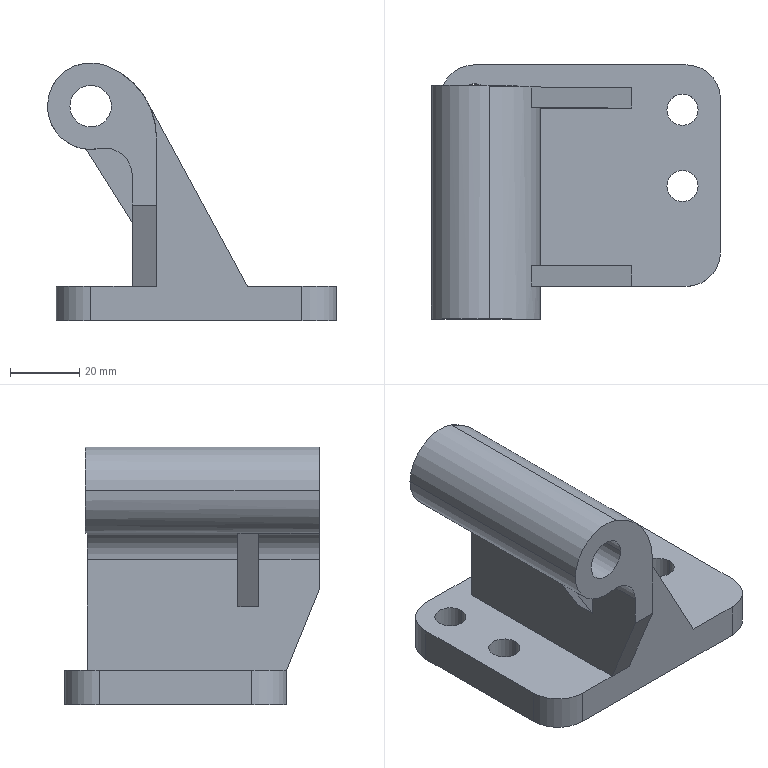Part | SolidWorks | features BaseBody 1 | 1 solid | 39 faces | box 83.5 x 73.5 x 74.5 mm | volume 109761 mm3 | plane 20 | cylinder 19 | commonest cylinder face diameters 9 x8 20 x4 12 x2 16 x2 25 x2 44.504 x1
STEP:
#1=CARTESIAN_POINT('',(5.5,32.,10.));
#2=VERTEX_POINT('',#1);
#3=CARTESIAN_POINT('',(14.5,32.,10.));
#4=VERTEX_POINT('',#3);
#5=CARTESIAN_POINT('',(10.,32.,10.));
#6=DIRECTION('',(0.,0.,-1.));
#7=DIRECTION('',(-1.,0.,0.));
#8=AXIS2_PLACEMENT_3D('',#5,#6,#7);
#9=CIRCLE('',#8,4.5);
#10=EDGE_CURVE('',#2,#4,#9,.T.);
#11=ORIENTED_EDGE('',*,*,#10,.F.);
#12=CARTESIAN_POINT('',(5.5,32.,0.));
#13=VERTEX_POINT('',#12);
#14=CARTESIAN_POINT('',(5.5,32.,10.));
#15=DIRECTION('',(0.,0.,-1.));
#16=VECTOR('',#15,1000.);
#17=LINE('',#14,#16);
#18=EDGE_CURVE('',#2,#13,#17,.T.);
#19=ORIENTED_EDGE('',*,*,#18,.T.);
#20=CARTESIAN_POINT('',(14.5,32.,0.));
#21=VERTEX_POINT('',#20);
#22=CARTESIAN_POINT('',(10.,32.,0.));
#23=DIRECTION('',(0.,0.,-1.));
#24=DIRECTION('',(-1.,0.,0.));
#25=AXIS2_PLACEMENT_3D('',#22,#23,#24);
#26=CIRCLE('',#25,4.5);
#27=EDGE_CURVE('',#13,#21,#26,.T.);
#28=ORIENTED_EDGE('',*,*,#27,.T.);
#29=CARTESIAN_POINT('',(14.5,32.,10.));
#30=DIRECTION('',(0.,0.,-1.));
#31=VECTOR('',#30,1000.);
#32=LINE('',#29,#31);
#33=EDGE_CURVE('',#4,#21,#32,.T.);
#34=ORIENTED_EDGE('',*,*,#33,.F.);
#35=EDGE_LOOP('',(#11,#19,#28,#34));
#36=FACE_OUTER_BOUND('',#35,.T.);
#37=CARTESIAN_POINT('',(10.,32.,10.));
#38=DIRECTION('',(0.,0.,-1.));
#39=DIRECTION('',(1.,0.,0.));
#40=AXIS2_PLACEMENT_3D('',#37,#38,#39);
#41=CYLINDRICAL_SURFACE('',#40,4.5);
#42=ADVANCED_FACE('',(#36),#41,.F.);
#43=CARTESIAN_POINT('',(5.5,54.,10.));
#44=VERTEX_POINT('',#43);
#45=CARTESIAN_POINT('',(14.5,54.,10.));
#46=VERTEX_POINT('',#45);
#47=CARTESIAN_POINT('',(10.,54.,10.));
#48=DIRECTION('',(0.,0.,-1.));
#49=DIRECTION('',(-1.,0.,0.));
#50=AXIS2_PLACEMENT_3D('',#47,#48,#49);
#51=CIRCLE('',#50,4.5);
#52=EDGE_CURVE('',#44,#46,#51,.T.);
#53=ORIENTED_EDGE('',*,*,#52,.F.);
#54=CARTESIAN_POINT('',(5.5,54.,0.));
#55=VERTEX_POINT('',#54);
#56=CARTESIAN_POINT('',(5.5,54.,10.));
#57=DIRECTION('',(0.,0.,-1.));
#58=VECTOR('',#57,1000.);
#59=LINE('',#56,#58);
#60=EDGE_CURVE('',#44,#55,#59,.T.);
#61=ORIENTED_EDGE('',*,*,#60,.T.);
#62=CARTESIAN_POINT('',(14.5,54.,0.));
#63=VERTEX_POINT('',#62);
#64=CARTESIAN_POINT('',(10.,54.,0.));
#65=DIRECTION('',(0.,0.,-1.));
#66=DIRECTION('',(-1.,0.,0.));
#67=AXIS2_PLACEMENT_3D('',#64,#65,#66);
#68=CIRCLE('',#67,4.5);
#69=EDGE_CURVE('',#55,#63,#68,.T.);
#70=ORIENTED_EDGE('',*,*,#69,.T.);
#71=CARTESIAN_POINT('',(14.5,54.,10.));
#72=DIRECTION('',(0.,0.,-1.));
#73=VECTOR('',#72,1000.);
#74=LINE('',#71,#73);
#75=EDGE_CURVE('',#46,#63,#74,.T.);
#76=ORIENTED_EDGE('',*,*,#75,.F.);
#77=EDGE_LOOP('',(#53,#61,#70,#76));
#78=FACE_OUTER_BOUND('',#77,.T.);
#79=CARTESIAN_POINT('',(10.,54.,10.));
#80=DIRECTION('',(0.,0.,-1.));
#81=DIRECTION('',(1.,0.,0.));
#82=AXIS2_PLACEMENT_3D('',#79,#80,#81);
#83=CYLINDRICAL_SURFACE('',#82,4.5);
#84=ADVANCED_FACE('',(#78),#83,.F.);
#85=CARTESIAN_POINT('',(22.5,58.,62.));
#86=VERTEX_POINT('',#85);
#87=CARTESIAN_POINT('',(-2.5,58.,62.));
#88=VERTEX_POINT('',#87);
#89=CARTESIAN_POINT('',(10.,58.,62.));
#90=DIRECTION('',(0.,1.,0.));
#91=DIRECTION('',(0.,0.,-1.));
#92=AXIS2_PLACEMENT_3D('',#89,#90,#91);
#93=CIRCLE('',#92,12.5);
#94=EDGE_CURVE('',#86,#88,#93,.T.);
#95=ORIENTED_EDGE('',*,*,#94,.F.);
#96=CARTESIAN_POINT('',(22.5,57.5,62.));
#97=VERTEX_POINT('',#96);
#98=CARTESIAN_POINT('',(22.5,57.5,62.));
#99=DIRECTION('',(0.,-1.,0.));
#100=VECTOR('',#99,1000.);
#101=LINE('',#98,#100);
#102=EDGE_CURVE('',#86,#97,#101,.T.);
#103=ORIENTED_EDGE('',*,*,#102,.T.);
#104=CARTESIAN_POINT('',(12.439,57.5,49.74));
#105=VERTEX_POINT('',#104);
#106=CARTESIAN_POINT('',(10.,57.5,62.));
#107=DIRECTION('',(0.,-1.,0.));
#108=DIRECTION('',(0.,0.,-1.));
#109=AXIS2_PLACEMENT_3D('',#106,#107,#108);
#110=CIRCLE('',#109,12.5);
#111=EDGE_CURVE('',#105,#97,#110,.T.);
#112=ORIENTED_EDGE('',*,*,#111,.F.);
#113=CARTESIAN_POINT('',(12.439,14.,49.74));
#114=VERTEX_POINT('',#113);
#115=CARTESIAN_POINT('',(12.439,-9.5,49.74));
#116=DIRECTION('',(0.,1.,0.));
#117=VECTOR('',#116,1000.);
#118=LINE('',#115,#117);
#119=EDGE_CURVE('',#114,#105,#118,.T.);
#120=ORIENTED_EDGE('',*,*,#119,.F.);
#121=CARTESIAN_POINT('',(8.698,14.,49.568));
#122=VERTEX_POINT('',#121);
#123=CARTESIAN_POINT('',(10.,14.,62.));
#124=DIRECTION('',(0.,-1.,0.));
#125=DIRECTION('',(0.,0.,1.));
#126=AXIS2_PLACEMENT_3D('',#123,#124,#125);
#127=CIRCLE('',#126,12.5);
#128=EDGE_CURVE('',#122,#114,#127,.T.);
#129=ORIENTED_EDGE('',*,*,#128,.F.);
#130=CARTESIAN_POINT('',(8.698,8.,49.568));
#131=VERTEX_POINT('',#130);
#132=CARTESIAN_POINT('',(8.698,57.5,49.568));
#133=DIRECTION('',(0.,-1.,0.));
#134=VECTOR('',#133,1000.);
#135=LINE('',#132,#134);
#136=EDGE_CURVE('',#122,#131,#135,.T.);
#137=ORIENTED_EDGE('',*,*,#136,.T.);
#138=CARTESIAN_POINT('',(12.439,8.,49.74));
#139=VERTEX_POINT('',#138);
#140=CARTESIAN_POINT('',(10.,8.,62.));
#141=DIRECTION('',(0.,-1.,0.));
#142=DIRECTION('',(0.,0.,1.));
#143=AXIS2_PLACEMENT_3D('',#140,#141,#142);
#144=CIRCLE('',#143,12.5);
#145=EDGE_CURVE('',#131,#139,#144,.T.);
#146=ORIENTED_EDGE('',*,*,#145,.T.);
#147=CARTESIAN_POINT('',(12.439,-9.5,49.74));
#148=VERTEX_POINT('',#147);
#149=CARTESIAN_POINT('',(12.439,-9.5,49.74));
#150=DIRECTION('',(0.,1.,0.));
#151=VECTOR('',#150,1000.);
#152=LINE('',#149,#151);
#153=EDGE_CURVE('',#148,#139,#152,.T.);
#154=ORIENTED_EDGE('',*,*,#153,.F.);
#155=CARTESIAN_POINT('',(-2.5,-9.5,62.));
#156=VERTEX_POINT('',#155);
#157=CARTESIAN_POINT('',(10.,-9.5,62.));
#158=DIRECTION('',(0.,1.,0.));
#159=DIRECTION('',(0.,0.,1.));
#160=AXIS2_PLACEMENT_3D('',#157,#158,#159);
#161=CIRCLE('',#160,12.5);
#162=EDGE_CURVE('',#148,#156,#161,.T.);
#163=ORIENTED_EDGE('',*,*,#162,.T.);
#164=CARTESIAN_POINT('',(-2.5,57.5,62.));
#165=DIRECTION('',(0.,-1.,0.));
#166=VECTOR('',#165,1000.);
#167=LINE('',#164,#166);
#168=EDGE_CURVE('',#88,#156,#167,.T.);
#169=ORIENTED_EDGE('',*,*,#168,.F.);
#170=EDGE_LOOP('',(#95,#103,#112,#120,#129,#137,#146,#154,#163,#169));
#171=FACE_OUTER_BOUND('',#170,.T.);
#172=CARTESIAN_POINT('',(10.,57.5,62.));
#173=DIRECTION('',(0.,-1.,0.));
#174=DIRECTION('',(-1.,0.,0.));
#175=AXIS2_PLACEMENT_3D('',#172,#173,#174);
#176=CYLINDRICAL_SURFACE('',#175,12.5);
#177=ADVANCED_FACE('',(#171),#176,.T.);
#178=CARTESIAN_POINT('',(4.,58.,62.));
#179=VERTEX_POINT('',#178);
#180=CARTESIAN_POINT('',(16.,58.,62.));
#181=VERTEX_POINT('',#180);
#182=CARTESIAN_POINT('',(10.,58.,62.));
#183=DIRECTION('',(0.,1.,0.));
#184=DIRECTION('',(0.,0.,-1.));
#185=AXIS2_PLACEMENT_3D('',#182,#183,#184);
#186=CIRCLE('',#185,6.);
#187=EDGE_CURVE('',#179,#181,#186,.T.);
#188=ORIENTED_EDGE('',*,*,#187,.T.);
#189=CARTESIAN_POINT('',(16.,-9.5,62.));
#190=VERTEX_POINT('',#189);
#191=CARTESIAN_POINT('',(16.,57.5,62.));
#192=DIRECTION('',(0.,-1.,0.));
#193=VECTOR('',#192,1000.);
#194=LINE('',#191,#193);
#195=EDGE_CURVE('',#181,#190,#194,.T.);
#196=ORIENTED_EDGE('',*,*,#195,.T.);
#197=CARTESIAN_POINT('',(4.,-9.5,62.));
#198=VERTEX_POINT('',#197);
#199=CARTESIAN_POINT('',(10.,-9.5,62.));
#200=DIRECTION('',(0.,1.,0.));
#201=DIRECTION('',(0.,0.,1.));
#202=AXIS2_PLACEMENT_3D('',#199,#200,#201);
#203=CIRCLE('',#202,6.);
#204=EDGE_CURVE('',#198,#190,#203,.T.);
#205=ORIENTED_EDGE('',*,*,#204,.F.);
#206=CARTESIAN_POINT('',(4.,57.5,62.));
#207=DIRECTION('',(0.,-1.,0.));
#208=VECTOR('',#207,1000.);
#209=LINE('',#206,#208);
#210=EDGE_CURVE('',#179,#198,#209,.T.);
#211=ORIENTED_EDGE('',*,*,#210,.F.);
#212=EDGE_LOOP('',(#188,#196,#205,#211));
#213=FACE_OUTER_BOUND('',#212,.T.);
#214=CARTESIAN_POINT('',(10.,57.5,62.));
#215=DIRECTION('',(0.,-1.,0.));
#216=DIRECTION('',(-1.,0.,0.));
#217=AXIS2_PLACEMENT_3D('',#214,#215,#216);
#218=CYLINDRICAL_SURFACE('',#217,6.);
#219=ADVANCED_FACE('',(#213),#218,.F.);
#220=CARTESIAN_POINT('',(65.5,29.,10.));
#221=VERTEX_POINT('',#220);
#222=CARTESIAN_POINT('',(74.5,29.,10.));
#223=VERTEX_POINT('',#222);
#224=CARTESIAN_POINT('',(70.,29.,10.));
#225=DIRECTION('',(0.,0.,-1.));
#226=DIRECTION('',(-1.,0.,0.));
#227=AXIS2_PLACEMENT_3D('',#224,#225,#226);
#228=CIRCLE('',#227,4.5);
#229=EDGE_CURVE('',#221,#223,#228,.T.);
#230=ORIENTED_EDGE('',*,*,#229,.F.);
#231=CARTESIAN_POINT('',(65.5,29.,0.));
#232=VERTEX_POINT('',#231);
#233=CARTESIAN_POINT('',(65.5,29.,20.));
#234=DIRECTION('',(0.,0.,-1.));
#235=VECTOR('',#234,1000.);
#236=LINE('',#233,#235);
#237=EDGE_CURVE('',#221,#232,#236,.T.);
#238=ORIENTED_EDGE('',*,*,#237,.T.);
#239=CARTESIAN_POINT('',(74.5,29.,0.));
#240=VERTEX_POINT('',#239);
#241=CARTESIAN_POINT('',(70.,29.,0.));
#242=DIRECTION('',(0.,0.,-1.));
#243=DIRECTION('',(-1.,0.,0.));
#244=AXIS2_PLACEMENT_3D('',#241,#242,#243);
#245=CIRCLE('',#244,4.5);
#246=EDGE_CURVE('',#232,#240,#245,.T.);
#247=ORIENTED_EDGE('',*,*,#246,.T.);
#248=CARTESIAN_POINT('',(74.5,29.,20.));
#249=DIRECTION('',(0.,0.,-1.));
#250=VECTOR('',#249,1000.);
#251=LINE('',#248,#250);
#252=EDGE_CURVE('',#223,#240,#251,.T.);
#253=ORIENTED_EDGE('',*,*,#252,.F.);
#254=EDGE_LOOP('',(#230,#238,#247,#253));
#255=FACE_OUTER_BOUND('',#254,.T.);
#256=CARTESIAN_POINT('',(70.,29.,20.));
#257=DIRECTION('',(0.,0.,-1.));
#258=DIRECTION('',(1.,0.,0.));
#259=AXIS2_PLACEMENT_3D('',#256,#257,#258);
#260=CYLINDRICAL_SURFACE('',#259,4.5);
#261=ADVANCED_FACE('',(#255),#260,.F.);
#262=CARTESIAN_POINT('',(65.5,51.,10.));
#263=VERTEX_POINT('',#262);
#264=CARTESIAN_POINT('',(74.5,51.,10.));
#265=VERTEX_POINT('',#264);
#266=CARTESIAN_POINT('',(70.,51.,10.));
#267=DIRECTION('',(0.,0.,-1.));
#268=DIRECTION('',(-1.,0.,0.));
#269=AXIS2_PLACEMENT_3D('',#266,#267,#268);
#270=CIRCLE('',#269,4.5);
#271=EDGE_CURVE('',#263,#265,#270,.T.);
#272=ORIENTED_EDGE('',*,*,#271,.F.);
#273=CARTESIAN_POINT('',(65.5,51.,0.));
#274=VERTEX_POINT('',#273);
#275=CARTESIAN_POINT('',(65.5,51.,20.));
#276=DIRECTION('',(0.,0.,-1.));
#277=VECTOR('',#276,1000.);
#278=LINE('',#275,#277);
#279=EDGE_CURVE('',#263,#274,#278,.T.);
#280=ORIENTED_EDGE('',*,*,#279,.T.);
#281=CARTESIAN_POINT('',(74.5,51.,0.));
#282=VERTEX_POINT('',#281);
#283=CARTESIAN_POINT('',(70.,51.,0.));
#284=DIRECTION('',(0.,0.,-1.));
#285=DIRECTION('',(-1.,0.,0.));
#286=AXIS2_PLACEMENT_3D('',#283,#284,#285);
#287=CIRCLE('',#286,4.5);
#288=EDGE_CURVE('',#274,#282,#287,.T.);
#289=ORIENTED_EDGE('',*,*,#288,.T.);
#290=CARTESIAN_POINT('',(74.5,51.,20.));
#291=DIRECTION('',(0.,0.,-1.));
#292=VECTOR('',#291,1000.);
#293=LINE('',#290,#292);
#294=EDGE_CURVE('',#265,#282,#293,.T.);
#295=ORIENTED_EDGE('',*,*,#294,.F.);
#296=EDGE_LOOP('',(#272,#280,#289,#295));
#297=FACE_OUTER_BOUND('',#296,.T.);
#298=CARTESIAN_POINT('',(70.,51.,20.));
#299=DIRECTION('',(0.,0.,-1.));
#300=DIRECTION('',(1.,0.,0.));
#301=AXIS2_PLACEMENT_3D('',#298,#299,#300);
#302=CYLINDRICAL_SURFACE('',#301,4.5);
#303=ADVANCED_FACE('',(#297),#302,.F.);
#304=ORIENTED_EDGE('',*,*,#187,.F.);
#305=CARTESIAN_POINT('',(10.,58.,62.));
#306=DIRECTION('',(0.,1.,0.));
#307=DIRECTION('',(0.,0.,-1.));
#308=AXIS2_PLACEMENT_3D('',#305,#306,#307);
#309=CIRCLE('',#308,6.);
#310=EDGE_CURVE('',#181,#179,#309,.T.);
#311=ORIENTED_EDGE('',*,*,#310,.F.);
#312=EDGE_LOOP('',(#304,#311));
#313=FACE_BOUND('',#312,.T.);
#314=CARTESIAN_POINT('',(10.,58.,62.));
#315=DIRECTION('',(0.,1.,0.));
#316=DIRECTION('',(0.,0.,-1.));
#317=AXIS2_PLACEMENT_3D('',#314,#315,#316);
#318=CIRCLE('',#317,12.5);
#319=EDGE_CURVE('',#88,#86,#318,.T.);
#320=ORIENTED_EDGE('',*,*,#319,.T.);
#321=ORIENTED_EDGE('',*,*,#94,.T.);
#322=EDGE_LOOP('',(#320,#321));
#323=FACE_OUTER_BOUND('',#322,.T.);
#324=CARTESIAN_POINT('',(10.,58.,62.));
#325=DIRECTION('',(0.,1.,0.));
#326=DIRECTION('',(1.,0.,0.));
#327=AXIS2_PLACEMENT_3D('',#324,#325,#326);
#328=PLANE('',#327);
#329=ADVANCED_FACE('',(#313,#323),#328,.T.);
#330=CARTESIAN_POINT('',(81.,54.,10.));
#331=VERTEX_POINT('',#330);
#332=CARTESIAN_POINT('',(71.,64.,10.));
#333=VERTEX_POINT('',#332);
#334=CARTESIAN_POINT('',(71.,54.,10.));
#335=DIRECTION('',(0.,0.,1.));
#336=DIRECTION('',(-1.,0.,0.));
#337=AXIS2_PLACEMENT_3D('',#334,#335,#336);
#338=CIRCLE('',#337,10.);
#339=EDGE_CURVE('',#331,#333,#338,.T.);
#340=ORIENTED_EDGE('',*,*,#339,.F.);
#341=CARTESIAN_POINT('',(81.,54.,0.));
#342=VERTEX_POINT('',#341);
#343=CARTESIAN_POINT('',(81.,54.,10.));
#344=DIRECTION('',(0.,0.,1.));
#345=VECTOR('',#344,1000.);
#346=LINE('',#343,#345);
#347=EDGE_CURVE('',#342,#331,#346,.T.);
#348=ORIENTED_EDGE('',*,*,#347,.F.);
#349=CARTESIAN_POINT('',(71.,64.,0.));
#350=VERTEX_POINT('',#349);
#351=CARTESIAN_POINT('',(71.,54.,0.));
#352=DIRECTION('',(0.,0.,-1.));
#353=DIRECTION('',(-1.,0.,0.));
#354=AXIS2_PLACEMENT_3D('',#351,#352,#353);
#355=CIRCLE('',#354,10.);
#356=EDGE_CURVE('',#350,#342,#355,.T.);
#357=ORIENTED_EDGE('',*,*,#356,.F.);
#358=CARTESIAN_POINT('',(71.,64.,10.));
#359=DIRECTION('',(0.,0.,-1.));
#360=VECTOR('',#359,1000.);
#361=LINE('',#358,#360);
#362=EDGE_CURVE('',#333,#350,#361,.T.);
#363=ORIENTED_EDGE('',*,*,#362,.F.);
#364=EDGE_LOOP('',(#340,#348,#357,#363));
#365=FACE_OUTER_BOUND('',#364,.T.);
#366=CARTESIAN_POINT('',(71.,54.,10.));
#367=DIRECTION('',(0.,0.,-1.));
#368=DIRECTION('',(1.,0.,0.));
#369=AXIS2_PLACEMENT_3D('',#366,#367,#368);
#370=CYLINDRICAL_SURFACE('',#369,10.);
#371=ADVANCED_FACE('',(#365),#370,.T.);
#372=CARTESIAN_POINT('',(71.,0.,10.));
#373=VERTEX_POINT('',#372);
#374=CARTESIAN_POINT('',(81.,10.,10.));
#375=VERTEX_POINT('',#374);
#376=CARTESIAN_POINT('',(71.,10.,10.));
#377=DIRECTION('',(0.,0.,1.));
#378=DIRECTION('',(-1.,0.,0.));
#379=AXIS2_PLACEMENT_3D('',#376,#377,#378);
#380=CIRCLE('',#379,10.);
#381=EDGE_CURVE('',#373,#375,#380,.T.);
#382=ORIENTED_EDGE('',*,*,#381,.F.);
#383=CARTESIAN_POINT('',(71.,0.,0.));
#384=VERTEX_POINT('',#383);
#385=CARTESIAN_POINT('',(71.,0.,10.));
#386=DIRECTION('',(0.,0.,1.));
#387=VECTOR('',#386,1000.);
#388=LINE('',#385,#387);
#389=EDGE_CURVE('',#384,#373,#388,.T.);
#390=ORIENTED_EDGE('',*,*,#389,.F.);
#391=CARTESIAN_POINT('',(81.,10.,0.));
#392=VERTEX_POINT('',#391);
#393=CARTESIAN_POINT('',(71.,10.,0.));
#394=DIRECTION('',(0.,0.,-1.));
#395=DIRECTION('',(-1.,0.,0.));
#396=AXIS2_PLACEMENT_3D('',#393,#394,#395);
#397=CIRCLE('',#396,10.);
#398=EDGE_CURVE('',#392,#384,#397,.T.);
#399=ORIENTED_EDGE('',*,*,#398,.F.);
#400=CARTESIAN_POINT('',(81.,10.,10.));
#401=DIRECTION('',(0.,0.,-1.));
#402=VECTOR('',#401,1000.);
#403=LINE('',#400,#402);
#404=EDGE_CURVE('',#375,#392,#403,.T.);
#405=ORIENTED_EDGE('',*,*,#404,.F.);
#406=EDGE_LOOP('',(#382,#390,#399,#405));
#407=FACE_OUTER_BOUND('',#406,.T.);
#408=CARTESIAN_POINT('',(71.,10.,10.));
#409=DIRECTION('',(0.,0.,-1.));
#410=DIRECTION('',(1.,0.,0.));
#411=AXIS2_PLACEMENT_3D('',#408,#409,#410);
#412=CYLINDRICAL_SURFACE('',#411,10.);
#413=ADVANCED_FACE('',(#407),#412,.T.);
#414=CARTESIAN_POINT('',(10.,64.,10.));
#415=VERTEX_POINT('',#414);
#416=CARTESIAN_POINT('',(0.,54.,10.));
#417=VERTEX_POINT('',#416);
#418=CARTESIAN_POINT('',(10.,54.,10.));
#419=DIRECTION('',(0.,0.,1.));
#420=DIRECTION('',(-1.,0.,0.));
#421=AXIS2_PLACEMENT_3D('',#418,#419,#420);
#422=CIRCLE('',#421,10.);
#423=EDGE_CURVE('',#415,#417,#422,.T.);
#424=ORIENTED_EDGE('',*,*,#423,.F.);
#425=CARTESIAN_POINT('',(10.,64.,0.));
#426=VERTEX_POINT('',#425);
#427=CARTESIAN_POINT('',(10.,64.,10.));
#428=DIRECTION('',(0.,0.,1.));
#429=VECTOR('',#428,1000.);
#430=LINE('',#427,#429);
#431=EDGE_CURVE('',#426,#415,#430,.T.);
#432=ORIENTED_EDGE('',*,*,#431,.F.);
#433=CARTESIAN_POINT('',(0.,54.,0.));
#434=VERTEX_POINT('',#433);
#435=CARTESIAN_POINT('',(10.,54.,0.));
#436=DIRECTION('',(0.,0.,-1.));
#437=DIRECTION('',(-1.,0.,0.));
#438=AXIS2_PLACEMENT_3D('',#435,#436,#437);
#439=CIRCLE('',#438,10.);
#440=EDGE_CURVE('',#434,#426,#439,.T.);
#441=ORIENTED_EDGE('',*,*,#440,.F.);
#442=CARTESIAN_POINT('',(0.,54.,10.));
#443=DIRECTION('',(0.,0.,-1.));
#444=VECTOR('',#443,1000.);
#445=LINE('',#442,#444);
#446=EDGE_CURVE('',#417,#434,#445,.T.);
#447=ORIENTED_EDGE('',*,*,#446,.F.);
#448=EDGE_LOOP('',(#424,#432,#441,#447));
#449=FACE_OUTER_BOUND('',#448,.T.);
#450=CARTESIAN_POINT('',(10.,54.,10.));
#451=DIRECTION('',(0.,0.,-1.));
#452=DIRECTION('',(1.,0.,0.));
#453=AXIS2_PLACEMENT_3D('',#450,#451,#452);
#454=CYLINDRICAL_SURFACE('',#453,10.);
#455=ADVANCED_FACE('',(#449),#454,.T.);
#456=CARTESIAN_POINT('',(0.,10.,10.));
#457=VERTEX_POINT('',#456);
#458=CARTESIAN_POINT('',(10.,0.,10.));
#459=VERTEX_POINT('',#458);
#460=CARTESIAN_POINT('',(10.,10.,10.));
#461=DIRECTION('',(0.,0.,1.));
#462=DIRECTION('',(-1.,0.,0.));
#463=AXIS2_PLACEMENT_3D('',#460,#461,#462);
#464=CIRCLE('',#463,10.);
#465=EDGE_CURVE('',#457,#459,#464,.T.);
#466=ORIENTED_EDGE('',*,*,#465,.F.);
#467=CARTESIAN_POINT('',(0.,10.,0.));
#468=VERTEX_POINT('',#467);
#469=CARTESIAN_POINT('',(0.,10.,10.));
#470=DIRECTION('',(0.,0.,1.));
#471=VECTOR('',#470,1000.);
#472=LINE('',#469,#471);
#473=EDGE_CURVE('',#468,#457,#472,.T.);
#474=ORIENTED_EDGE('',*,*,#473,.F.);
#475=CARTESIAN_POINT('',(10.,0.,0.));
#476=VERTEX_POINT('',#475);
#477=CARTESIAN_POINT('',(10.,10.,0.));
#478=DIRECTION('',(0.,0.,-1.));
#479=DIRECTION('',(-1.,0.,0.));
#480=AXIS2_PLACEMENT_3D('',#477,#478,#479);
#481=CIRCLE('',#480,10.);
#482=EDGE_CURVE('',#476,#468,#481,.T.);
#483=ORIENTED_EDGE('',*,*,#482,.F.);
#484=CARTESIAN_POINT('',(10.,0.,10.));
#485=DIRECTION('',(0.,0.,-1.));
#486=VECTOR('',#485,1000.);
#487=LINE('',#484,#486);
#488=EDGE_CURVE('',#459,#476,#487,.T.);
#489=ORIENTED_EDGE('',*,*,#488,.F.);
#490=EDGE_LOOP('',(#466,#474,#483,#489));
#491=FACE_OUTER_BOUND('',#490,.T.);
#492=CARTESIAN_POINT('',(10.,10.,10.));
#493=DIRECTION('',(0.,0.,-1.));
#494=DIRECTION('',(1.,0.,0.));
#495=AXIS2_PLACEMENT_3D('',#492,#493,#494);
#496=CYLINDRICAL_SURFACE('',#495,10.);
#497=ADVANCED_FACE('',(#491),#496,.T.);
#498=ORIENTED_EDGE('',*,*,#279,.F.);
#499=CARTESIAN_POINT('',(70.,51.,10.));
#500=DIRECTION('',(0.,0.,-1.));
#501=DIRECTION('',(-1.,0.,0.));
#502=AXIS2_PLACEMENT_3D('',#499,#500,#501);
#503=CIRCLE('',#502,4.5);
#504=EDGE_CURVE('',#265,#263,#503,.T.);
#505=ORIENTED_EDGE('',*,*,#504,.F.);
#506=ORIENTED_EDGE('',*,*,#294,.T.);
#507=CARTESIAN_POINT('',(70.,51.,0.));
#508=DIRECTION('',(0.,0.,-1.));
#509=DIRECTION('',(-1.,0.,0.));
#510=AXIS2_PLACEMENT_3D('',#507,#508,#509);
#511=CIRCLE('',#510,4.5);
#512=EDGE_CURVE('',#282,#274,#511,.T.);
#513=ORIENTED_EDGE('',*,*,#512,.T.);
#514=EDGE_LOOP('',(#498,#505,#506,#513));
#515=FACE_OUTER_BOUND('',#514,.T.);
#516=CARTESIAN_POINT('',(70.,51.,20.));
#517=DIRECTION('',(0.,0.,-1.));
#518=DIRECTION('',(1.,0.,0.));
#519=AXIS2_PLACEMENT_3D('',#516,#517,#518);
#520=CYLINDRICAL_SURFACE('',#519,4.5);
#521=ADVANCED_FACE('',(#515),#520,.F.);
#522=ORIENTED_EDGE('',*,*,#237,.F.);
#523=CARTESIAN_POINT('',(70.,29.,10.));
#524=DIRECTION('',(0.,0.,-1.));
#525=DIRECTION('',(-1.,0.,0.));
#526=AXIS2_PLACEMENT_3D('',#523,#524,#525);
#527=CIRCLE('',#526,4.5);
#528=EDGE_CURVE('',#223,#221,#527,.T.);
#529=ORIENTED_EDGE('',*,*,#528,.F.);
#530=ORIENTED_EDGE('',*,*,#252,.T.);
#531=CARTESIAN_POINT('',(70.,29.,0.));
#532=DIRECTION('',(0.,0.,-1.));
#533=DIRECTION('',(-1.,0.,0.));
#534=AXIS2_PLACEMENT_3D('',#531,#532,#533);
#535=CIRCLE('',#534,4.5);
#536=EDGE_CURVE('',#240,#232,#535,.T.);
#537=ORIENTED_EDGE('',*,*,#536,.T.);
#538=EDGE_LOOP('',(#522,#529,#530,#537));
#539=FACE_OUTER_BOUND('',#538,.T.);
#540=CARTESIAN_POINT('',(70.,29.,20.));
#541=DIRECTION('',(0.,0.,-1.));
#542=DIRECTION('',(1.,0.,0.));
#543=AXIS2_PLACEMENT_3D('',#540,#541,#542);
#544=CYLINDRICAL_SURFACE('',#543,4.5);
#545=ADVANCED_FACE('',(#539),#544,.F.);
#546=ORIENTED_EDGE('',*,*,#128,.T.);
#547=CARTESIAN_POINT('',(22.,14.,41.894));
#548=VERTEX_POINT('',#547);
#549=CARTESIAN_POINT('',(14.,14.,41.894));
#550=DIRECTION('',(0.,1.,0.));
#551=DIRECTION('',(0.,0.,1.));
#552=AXIS2_PLACEMENT_3D('',#549,#550,#551);
#553=CIRCLE('',#552,8.);
#554=EDGE_CURVE('',#114,#548,#553,.T.);
#555=ORIENTED_EDGE('',*,*,#554,.T.);
#556=CARTESIAN_POINT('',(22.,14.,28.309));
#557=VERTEX_POINT('',#556);
#558=CARTESIAN_POINT('',(22.,14.,50.4));
#559=DIRECTION('',(0.,0.,1.));
#560=VECTOR('',#559,1000.);
#561=LINE('',#558,#560);
#562=EDGE_CURVE('',#557,#548,#561,.T.);
#563=ORIENTED_EDGE('',*,*,#562,.F.);
#564=CARTESIAN_POINT('',(22.,14.,28.309));
#565=DIRECTION('',(0.5304,0.,-0.8477));
#566=VECTOR('',#565,1000.);
#567=LINE('',#564,#566);
#568=EDGE_CURVE('',#122,#557,#567,.T.);
#569=ORIENTED_EDGE('',*,*,#568,.F.);
#570=EDGE_LOOP('',(#546,#555,#563,#569));
#571=FACE_OUTER_BOUND('',#570,.T.);
#572=CARTESIAN_POINT('',(0.,14.,0.));
#573=DIRECTION('',(0.,1.,0.));
#574=DIRECTION('',(1.,0.,0.));
#575=AXIS2_PLACEMENT_3D('',#572,#573,#574);
#576=PLANE('',#575);
#577=ADVANCED_FACE('',(#571),#576,.T.);
#578=CARTESIAN_POINT('',(22.,8.,41.894));
#579=VERTEX_POINT('',#578);
#580=CARTESIAN_POINT('',(14.,8.,41.894));
#581=DIRECTION('',(0.,1.,0.));
#582=DIRECTION('',(0.,0.,1.));
#583=AXIS2_PLACEMENT_3D('',#580,#581,#582);
#584=CIRCLE('',#583,8.);
#585=EDGE_CURVE('',#139,#579,#584,.T.);
#586=ORIENTED_EDGE('',*,*,#585,.F.);
#587=ORIENTED_EDGE('',*,*,#145,.F.);
#588=CARTESIAN_POINT('',(22.,8.,28.309));
#589=VERTEX_POINT('',#588);
#590=CARTESIAN_POINT('',(22.,8.,28.309));
#591=DIRECTION('',(0.5304,0.,-0.8477));
#592=VECTOR('',#591,1000.);
#593=LINE('',#590,#592);
#594=EDGE_CURVE('',#131,#589,#593,.T.);
#595=ORIENTED_EDGE('',*,*,#594,.T.);
#596=CARTESIAN_POINT('',(22.,8.,50.4));
#597=DIRECTION('',(0.,0.,1.));
#598=VECTOR('',#597,1000.);
#599=LINE('',#596,#598);
#600=EDGE_CURVE('',#589,#579,#599,.T.);
#601=ORIENTED_EDGE('',*,*,#600,.T.);
#602=EDGE_LOOP('',(#586,#587,#595,#601));
#603=FACE_OUTER_BOUND('',#602,.T.);
#604=CARTESIAN_POINT('',(0.,8.,0.));
#605=DIRECTION('',(0.,1.,0.));
#606=DIRECTION('',(1.,0.,0.));
#607=AXIS2_PLACEMENT_3D('',#604,#605,#606);
#608=PLANE('',#607);
#609=ADVANCED_FACE('',(#603),#608,.F.);
#610=ORIENTED_EDGE('',*,*,#136,.F.);
#611=ORIENTED_EDGE('',*,*,#568,.T.);
#612=CARTESIAN_POINT('',(22.,8.,28.309));
#613=DIRECTION('',(0.,-1.,0.));
#614=VECTOR('',#613,1000.);
#615=LINE('',#612,#614);
#616=EDGE_CURVE('',#557,#589,#615,.T.);
#617=ORIENTED_EDGE('',*,*,#616,.T.);
#618=ORIENTED_EDGE('',*,*,#594,.F.);
#619=EDGE_LOOP('',(#610,#611,#617,#618));
#620=FACE_OUTER_BOUND('',#619,.T.);
#621=CARTESIAN_POINT('',(22.,8.,28.309));
#622=DIRECTION('',(-0.8477,0.,-0.5304));
#623=DIRECTION('',(-0.5304,0.,0.8477));
#624=AXIS2_PLACEMENT_3D('',#621,#622,#623);
#625=PLANE('',#624);
#626=ADVANCED_FACE('',(#620),#625,.T.);
#627=CARTESIAN_POINT('',(22.,-9.5,33.462));
#628=VERTEX_POINT('',#627);
#629=CARTESIAN_POINT('',(22.,0.,10.));
#630=VERTEX_POINT('',#629);
#631=CARTESIAN_POINT('',(22.,1.448,6.423));
#632=DIRECTION('',(0.,0.3753,-0.9269));
#633=VECTOR('',#632,1000.);
#634=LINE('',#631,#633);
#635=EDGE_CURVE('',#628,#630,#634,.T.);
#636=ORIENTED_EDGE('',*,*,#635,.T.);
#637=CARTESIAN_POINT('',(29.,0.,10.));
#638=VERTEX_POINT('',#637);
#639=CARTESIAN_POINT('',(-5.,0.,10.));
#640=DIRECTION('',(-1.,0.,0.));
#641=VECTOR('',#640,1000.);
#642=LINE('',#639,#641);
#643=EDGE_CURVE('',#638,#630,#642,.T.);
#644=ORIENTED_EDGE('',*,*,#643,.F.);
#645=CARTESIAN_POINT('',(29.,-9.5,33.462));
#646=VERTEX_POINT('',#645);
#647=CARTESIAN_POINT('',(29.,0.,10.));
#648=DIRECTION('',(0.,-0.3753,0.9269));
#649=VECTOR('',#648,1000.);
#650=LINE('',#647,#649);
#651=EDGE_CURVE('',#638,#646,#650,.T.);
#652=ORIENTED_EDGE('',*,*,#651,.T.);
#653=CARTESIAN_POINT('',(10.,-9.5,33.462));
#654=DIRECTION('',(1.,0.,0.));
#655=VECTOR('',#654,1000.);
#656=LINE('',#653,#655);
#657=EDGE_CURVE('',#628,#646,#656,.T.);
#658=ORIENTED_EDGE('',*,*,#657,.F.);
#659=EDGE_LOOP('',(#636,#644,#652,#658));
#660=FACE_OUTER_BOUND('',#659,.T.);
#661=CARTESIAN_POINT('',(-5.,0.,10.));
#662=DIRECTION('',(0.,0.9269,0.3753));
#663=DIRECTION('',(1.,0.,0.));
#664=AXIS2_PLACEMENT_3D('',#661,#662,#663);
#665=PLANE('',#664);
#666=ADVANCED_FACE('',(#660),#665,.F.);
#667=CARTESIAN_POINT('',(29.,0.,52.806));
#668=VERTEX_POINT('',#667);
#669=CARTESIAN_POINT('',(29.,0.,52.806));
#670=DIRECTION('',(0.,0.,-1.));
#671=VECTOR('',#670,1000.);
#672=LINE('',#669,#671);
#673=EDGE_CURVE('',#668,#638,#672,.T.);
#674=ORIENTED_EDGE('',*,*,#673,.F.);
#675=CARTESIAN_POINT('',(29.,-9.5,52.806));
#676=VERTEX_POINT('',#675);
#677=CARTESIAN_POINT('',(29.,-9.5,52.806));
#678=DIRECTION('',(0.,1.,0.));
#679=VECTOR('',#678,1000.);
#680=LINE('',#677,#679);
#681=EDGE_CURVE('',#676,#668,#680,.T.);
#682=ORIENTED_EDGE('',*,*,#681,.F.);
#683=CARTESIAN_POINT('',(29.,-9.5,52.806));
#684=DIRECTION('',(0.,0.,-1.));
#685=VECTOR('',#684,1000.);
#686=LINE('',#683,#685);
#687=EDGE_CURVE('',#676,#646,#686,.T.);
#688=ORIENTED_EDGE('',*,*,#687,.T.);
#689=ORIENTED_EDGE('',*,*,#651,.F.);
#690=EDGE_LOOP('',(#674,#682,#688,#689));
#691=FACE_OUTER_BOUND('',#690,.T.);
#692=CARTESIAN_POINT('',(29.,-9.5,52.806));
#693=DIRECTION('',(1.,0.,0.));
#694=DIRECTION('',(0.,0.,-1.));
#695=AXIS2_PLACEMENT_3D('',#692,#693,#694);
#696=PLANE('',#695);
#697=ADVANCED_FACE('',(#691),#696,.T.);
#698=ORIENTED_EDGE('',*,*,#554,.F.);
#699=ORIENTED_EDGE('',*,*,#119,.T.);
#700=CARTESIAN_POINT('',(22.,57.5,41.894));
#701=VERTEX_POINT('',#700);
#702=CARTESIAN_POINT('',(14.,57.5,41.894));
#703=DIRECTION('',(0.,-1.,0.));
#704=DIRECTION('',(1.,0.,0.));
#705=AXIS2_PLACEMENT_3D('',#702,#703,#704);
#706=CIRCLE('',#705,8.);
#707=EDGE_CURVE('',#701,#105,#706,.T.);
#708=ORIENTED_EDGE('',*,*,#707,.F.);
#709=CARTESIAN_POINT('',(22.,-9.5,41.894));
#710=DIRECTION('',(0.,1.,0.));
#711=VECTOR('',#710,1000.);
#712=LINE('',#709,#711);
#713=EDGE_CURVE('',#548,#701,#712,.T.);
#714=ORIENTED_EDGE('',*,*,#713,.F.);
#715=EDGE_LOOP('',(#698,#699,#708,#714));
#716=FACE_OUTER_BOUND('',#715,.T.);
#717=CARTESIAN_POINT('',(14.,-9.5,41.894));
#718=DIRECTION('',(0.,1.,0.));
#719=DIRECTION('',(0.,0.,-1.));
#720=AXIS2_PLACEMENT_3D('',#717,#718,#719);
#721=CYLINDRICAL_SURFACE('',#720,8.);
#722=ADVANCED_FACE('',(#716),#721,.F.);
#723=ORIENTED_EDGE('',*,*,#204,.T.);
#724=CARTESIAN_POINT('',(10.,-9.5,62.));
#725=DIRECTION('',(0.,1.,0.));
#726=DIRECTION('',(0.,0.,1.));
#727=AXIS2_PLACEMENT_3D('',#724,#725,#726);
#728=CIRCLE('',#727,6.);
#729=EDGE_CURVE('',#190,#198,#728,.T.);
#730=ORIENTED_EDGE('',*,*,#729,.T.);
#731=EDGE_LOOP('',(#723,#730));
#732=FACE_BOUND('',#731,.T.);
#733=CARTESIAN_POINT('',(22.,-9.5,41.894));
#734=VERTEX_POINT('',#733);
#735=CARTESIAN_POINT('',(22.,-9.5,1.99));
#736=DIRECTION('',(0.,0.,1.));
#737=VECTOR('',#736,1000.);
#738=LINE('',#735,#737);
#739=EDGE_CURVE('',#628,#734,#738,.T.);
#740=ORIENTED_EDGE('',*,*,#739,.F.);
#741=ORIENTED_EDGE('',*,*,#657,.T.);
#742=ORIENTED_EDGE('',*,*,#687,.F.);
#743=CARTESIAN_POINT('',(14.169,-9.5,73.784));
#744=VERTEX_POINT('',#743);
#745=CARTESIAN_POINT('',(6.748,-9.5,52.806));
#746=DIRECTION('',(0.,1.,0.));
#747=DIRECTION('',(1.,0.,0.));
#748=AXIS2_PLACEMENT_3D('',#745,#746,#747);
#749=CIRCLE('',#748,22.252);
#750=EDGE_CURVE('',#744,#676,#749,.T.);
#751=ORIENTED_EDGE('',*,*,#750,.F.);
#752=CARTESIAN_POINT('',(10.,-9.5,62.));
#753=DIRECTION('',(0.,1.,0.));
#754=DIRECTION('',(0.,0.,1.));
#755=AXIS2_PLACEMENT_3D('',#752,#753,#754);
#756=CIRCLE('',#755,12.5);
#757=EDGE_CURVE('',#156,#744,#756,.T.);
#758=ORIENTED_EDGE('',*,*,#757,.F.);
#759=ORIENTED_EDGE('',*,*,#162,.F.);
#760=CARTESIAN_POINT('',(14.,-9.5,41.894));
#761=DIRECTION('',(0.,-1.,0.));
#762=DIRECTION('',(1.,0.,0.));
#763=AXIS2_PLACEMENT_3D('',#760,#761,#762);
#764=CIRCLE('',#763,8.);
#765=EDGE_CURVE('',#734,#148,#764,.T.);
#766=ORIENTED_EDGE('',*,*,#765,.F.);
#767=EDGE_LOOP('',(#740,#741,#742,#751,#758,#759,#766));
#768=FACE_OUTER_BOUND('',#767,.T.);
#769=CARTESIAN_POINT('',(10.,-9.5,62.));
#770=DIRECTION('',(0.,1.,0.));
#771=DIRECTION('',(1.,0.,0.));
#772=AXIS2_PLACEMENT_3D('',#769,#770,#771);
#773=PLANE('',#772);
#774=ADVANCED_FACE('',(#732,#768),#773,.F.);
#775=ORIENTED_EDGE('',*,*,#195,.F.);
#776=ORIENTED_EDGE('',*,*,#310,.T.);
#777=ORIENTED_EDGE('',*,*,#210,.T.);
#778=ORIENTED_EDGE('',*,*,#729,.F.);
#779=EDGE_LOOP('',(#775,#776,#777,#778));
#780=FACE_OUTER_BOUND('',#779,.T.);
#781=CARTESIAN_POINT('',(10.,57.5,62.));
#782=DIRECTION('',(0.,-1.,0.));
#783=DIRECTION('',(-1.,0.,0.));
#784=AXIS2_PLACEMENT_3D('',#781,#782,#783);
#785=CYLINDRICAL_SURFACE('',#784,6.);
#786=ADVANCED_FACE('',(#780),#785,.F.);
#787=ORIENTED_EDGE('',*,*,#153,.T.);
#788=ORIENTED_EDGE('',*,*,#585,.T.);
#789=CARTESIAN_POINT('',(22.,-9.5,41.894));
#790=DIRECTION('',(0.,1.,0.));
#791=VECTOR('',#790,1000.);
#792=LINE('',#789,#791);
#793=EDGE_CURVE('',#734,#579,#792,.T.);
#794=ORIENTED_EDGE('',*,*,#793,.F.);
#795=ORIENTED_EDGE('',*,*,#765,.T.);
#796=EDGE_LOOP('',(#787,#788,#794,#795));
#797=FACE_OUTER_BOUND('',#796,.T.);
#798=CARTESIAN_POINT('',(14.,-9.5,41.894));
#799=DIRECTION('',(0.,1.,0.));
#800=DIRECTION('',(0.,0.,-1.));
#801=AXIS2_PLACEMENT_3D('',#798,#799,#800);
#802=CYLINDRICAL_SURFACE('',#801,8.);
#803=ADVANCED_FACE('',(#797),#802,.F.);
#804=ORIENTED_EDGE('',*,*,#102,.F.);
#805=ORIENTED_EDGE('',*,*,#319,.F.);
#806=ORIENTED_EDGE('',*,*,#168,.T.);
#807=ORIENTED_EDGE('',*,*,#757,.T.);
#808=CARTESIAN_POINT('',(14.169,57.5,73.784));
#809=VERTEX_POINT('',#808);
#810=CARTESIAN_POINT('',(14.169,-9.5,73.784));
#811=DIRECTION('',(0.,1.,0.));
#812=VECTOR('',#811,1000.);
#813=LINE('',#810,#812);
#814=EDGE_CURVE('',#744,#809,#813,.T.);
#815=ORIENTED_EDGE('',*,*,#814,.T.);
#816=CARTESIAN_POINT('',(10.,57.5,62.));
#817=DIRECTION('',(0.,-1.,0.));
#818=DIRECTION('',(0.,0.,-1.));
#819=AXIS2_PLACEMENT_3D('',#816,#817,#818);
#820=CIRCLE('',#819,12.5);
#821=EDGE_CURVE('',#97,#809,#820,.T.);
#822=ORIENTED_EDGE('',*,*,#821,.F.);
#823=EDGE_LOOP('',(#804,#805,#806,#807,#815,#822));
#824=FACE_OUTER_BOUND('',#823,.T.);
#825=CARTESIAN_POINT('',(10.,57.5,62.));
#826=DIRECTION('',(0.,-1.,0.));
#827=DIRECTION('',(-1.,0.,0.));
#828=AXIS2_PLACEMENT_3D('',#825,#826,#827);
#829=CYLINDRICAL_SURFACE('',#828,12.5);
#830=ADVANCED_FACE('',(#824),#829,.T.);
#831=CARTESIAN_POINT('',(26.306,6.,63.42));
#832=VERTEX_POINT('',#831);
#833=CARTESIAN_POINT('',(26.306,0.,63.42));
#834=VERTEX_POINT('',#833);
#835=CARTESIAN_POINT('',(26.306,6.,63.42));
#836=DIRECTION('',(0.,-1.,0.));
#837=VECTOR('',#836,1000.);
#838=LINE('',#835,#837);
#839=EDGE_CURVE('',#832,#834,#838,.T.);
#840=ORIENTED_EDGE('',*,*,#839,.F.);
#841=CARTESIAN_POINT('',(29.,6.,52.806));
#842=VERTEX_POINT('',#841);
#843=CARTESIAN_POINT('',(6.748,6.,52.806));
#844=DIRECTION('',(0.,1.,0.));
#845=DIRECTION('',(1.,0.,0.));
#846=AXIS2_PLACEMENT_3D('',#843,#844,#845);
#847=CIRCLE('',#846,22.252);
#848=EDGE_CURVE('',#832,#842,#847,.T.);
#849=ORIENTED_EDGE('',*,*,#848,.T.);
#850=CARTESIAN_POINT('',(29.,51.5,52.806));
#851=VERTEX_POINT('',#850);
#852=CARTESIAN_POINT('',(29.,-9.5,52.806));
#853=DIRECTION('',(0.,1.,0.));
#854=VECTOR('',#853,1000.);
#855=LINE('',#852,#854);
#856=EDGE_CURVE('',#842,#851,#855,.T.);
#857=ORIENTED_EDGE('',*,*,#856,.T.);
#858=CARTESIAN_POINT('',(26.306,51.5,63.42));
#859=VERTEX_POINT('',#858);
#860=CARTESIAN_POINT('',(6.748,51.5,52.806));
#861=DIRECTION('',(0.,1.,0.));
#862=DIRECTION('',(0.,0.,-1.));
#863=AXIS2_PLACEMENT_3D('',#860,#861,#862);
#864=CIRCLE('',#863,22.252);
#865=EDGE_CURVE('',#859,#851,#864,.T.);
#866=ORIENTED_EDGE('',*,*,#865,.F.);
#867=CARTESIAN_POINT('',(26.306,57.5,63.42));
#868=VERTEX_POINT('',#867);
#869=CARTESIAN_POINT('',(26.306,51.5,63.42));
#870=DIRECTION('',(0.,1.,0.));
#871=VECTOR('',#870,1000.);
#872=LINE('',#869,#871);
#873=EDGE_CURVE('',#859,#868,#872,.T.);
#874=ORIENTED_EDGE('',*,*,#873,.T.);
#875=CARTESIAN_POINT('',(6.748,57.5,52.806));
#876=DIRECTION('',(0.,1.,0.));
#877=DIRECTION('',(1.,0.,0.));
#878=AXIS2_PLACEMENT_3D('',#875,#876,#877);
#879=CIRCLE('',#878,22.252);
#880=EDGE_CURVE('',#809,#868,#879,.T.);
#881=ORIENTED_EDGE('',*,*,#880,.F.);
#882=ORIENTED_EDGE('',*,*,#814,.F.);
#883=ORIENTED_EDGE('',*,*,#750,.T.);
#884=ORIENTED_EDGE('',*,*,#681,.T.);
#885=CARTESIAN_POINT('',(6.748,0.,52.806));
#886=DIRECTION('',(0.,1.,0.));
#887=DIRECTION('',(1.,0.,0.));
#888=AXIS2_PLACEMENT_3D('',#885,#886,#887);
#889=CIRCLE('',#888,22.252);
#890=EDGE_CURVE('',#834,#668,#889,.T.);
#891=ORIENTED_EDGE('',*,*,#890,.F.);
#892=EDGE_LOOP('',(#840,#849,#857,#866,#874,#881,#882,#883,#884,#891));
#893=FACE_OUTER_BOUND('',#892,.T.);
#894=CARTESIAN_POINT('',(6.748,-9.5,52.806));
#895=DIRECTION('',(0.,1.,0.));
#896=DIRECTION('',(0.,0.,-1.));
#897=AXIS2_PLACEMENT_3D('',#894,#895,#896);
#898=CYLINDRICAL_SURFACE('',#897,22.252);
#899=ADVANCED_FACE('',(#893),#898,.T.);
#900=CARTESIAN_POINT('',(55.295,6.,10.));
#901=VERTEX_POINT('',#900);
#902=CARTESIAN_POINT('',(57.155,6.,6.573));
#903=DIRECTION('',(-0.477,0.,0.8789));
#904=VECTOR('',#903,1000.);
#905=LINE('',#902,#904);
#906=EDGE_CURVE('',#901,#832,#905,.T.);
#907=ORIENTED_EDGE('',*,*,#906,.F.);
#908=CARTESIAN_POINT('',(29.,6.,10.));
#909=VERTEX_POINT('',#908);
#910=CARTESIAN_POINT('',(0.,6.,10.));
#911=DIRECTION('',(-1.,0.,0.));
#912=VECTOR('',#911,1000.);
#913=LINE('',#910,#912);
#914=EDGE_CURVE('',#901,#909,#913,.T.);
#915=ORIENTED_EDGE('',*,*,#914,.T.);
#916=CARTESIAN_POINT('',(29.,6.,52.806));
#917=DIRECTION('',(0.,0.,-1.));
#918=VECTOR('',#917,1000.);
#919=LINE('',#916,#918);
#920=EDGE_CURVE('',#842,#909,#919,.T.);
#921=ORIENTED_EDGE('',*,*,#920,.F.);
#922=ORIENTED_EDGE('',*,*,#848,.F.);
#923=EDGE_LOOP('',(#907,#915,#921,#922));
#924=FACE_OUTER_BOUND('',#923,.T.);
#925=CARTESIAN_POINT('',(0.,6.,0.));
#926=DIRECTION('',(0.,-1.,0.));
#927=DIRECTION('',(-1.,0.,0.));
#928=AXIS2_PLACEMENT_3D('',#925,#926,#927);
#929=PLANE('',#928);
#930=ADVANCED_FACE('',(#924),#929,.F.);
#931=CARTESIAN_POINT('',(55.295,0.,10.));
#932=VERTEX_POINT('',#931);
#933=CARTESIAN_POINT('',(55.295,0.,10.));
#934=DIRECTION('',(0.,-1.,0.));
#935=VECTOR('',#934,1000.);
#936=LINE('',#933,#935);
#937=EDGE_CURVE('',#901,#932,#936,.T.);
#938=ORIENTED_EDGE('',*,*,#937,.F.);
#939=ORIENTED_EDGE('',*,*,#906,.T.);
#940=ORIENTED_EDGE('',*,*,#839,.T.);
#941=CARTESIAN_POINT('',(57.155,0.,6.573));
#942=DIRECTION('',(-0.477,0.,0.8789));
#943=VECTOR('',#942,1000.);
#944=LINE('',#941,#943);
#945=EDGE_CURVE('',#932,#834,#944,.T.);
#946=ORIENTED_EDGE('',*,*,#945,.F.);
#947=EDGE_LOOP('',(#938,#939,#940,#946));
#948=FACE_OUTER_BOUND('',#947,.T.);
#949=CARTESIAN_POINT('',(57.155,6.,6.573));
#950=DIRECTION('',(0.8789,0.,0.477));
#951=DIRECTION('',(0.,-1.,0.));
#952=AXIS2_PLACEMENT_3D('',#949,#950,#951);
#953=PLANE('',#952);
#954=ADVANCED_FACE('',(#948),#953,.T.);
#955=CARTESIAN_POINT('',(55.295,51.5,10.));
#956=VERTEX_POINT('',#955);
#957=CARTESIAN_POINT('',(29.,51.5,10.));
#958=VERTEX_POINT('',#957);
#959=CARTESIAN_POINT('',(0.,51.5,10.));
#960=DIRECTION('',(-1.,0.,0.));
#961=VECTOR('',#960,1000.);
#962=LINE('',#959,#961);
#963=EDGE_CURVE('',#956,#958,#962,.T.);
#964=ORIENTED_EDGE('',*,*,#963,.F.);
#965=CARTESIAN_POINT('',(26.306,51.5,63.42));
#966=DIRECTION('',(0.477,0.,-0.8789));
#967=VECTOR('',#966,1000.);
#968=LINE('',#965,#967);
#969=EDGE_CURVE('',#859,#956,#968,.T.);
#970=ORIENTED_EDGE('',*,*,#969,.F.);
#971=ORIENTED_EDGE('',*,*,#865,.T.);
#972=CARTESIAN_POINT('',(29.,51.5,52.806));
#973=DIRECTION('',(0.,0.,-1.));
#974=VECTOR('',#973,1000.);
#975=LINE('',#972,#974);
#976=EDGE_CURVE('',#851,#958,#975,.T.);
#977=ORIENTED_EDGE('',*,*,#976,.T.);
#978=EDGE_LOOP('',(#964,#970,#971,#977));
#979=FACE_OUTER_BOUND('',#978,.T.);
#980=CARTESIAN_POINT('',(0.,51.5,0.));
#981=DIRECTION('',(0.,-1.,0.));
#982=DIRECTION('',(0.,0.,-1.));
#983=AXIS2_PLACEMENT_3D('',#980,#981,#982);
#984=PLANE('',#983);
#985=ADVANCED_FACE('',(#979),#984,.T.);
#986=CARTESIAN_POINT('',(55.295,57.5,10.));
#987=VERTEX_POINT('',#986);
#988=CARTESIAN_POINT('',(55.295,0.,10.));
#989=DIRECTION('',(0.,-1.,0.));
#990=VECTOR('',#989,1000.);
#991=LINE('',#988,#990);
#992=EDGE_CURVE('',#987,#956,#991,.T.);
#993=ORIENTED_EDGE('',*,*,#992,.F.);
#994=CARTESIAN_POINT('',(26.306,57.5,63.42));
#995=DIRECTION('',(0.477,0.,-0.8789));
#996=VECTOR('',#995,1000.);
#997=LINE('',#994,#996);
#998=EDGE_CURVE('',#868,#987,#997,.T.);
#999=ORIENTED_EDGE('',*,*,#998,.F.);
#1000=ORIENTED_EDGE('',*,*,#873,.F.);
#1001=ORIENTED_EDGE('',*,*,#969,.T.);
#1002=EDGE_LOOP('',(#993,#999,#1000,#1001));
#1003=FACE_OUTER_BOUND('',#1002,.T.);
#1004=CARTESIAN_POINT('',(26.306,51.5,63.42));
#1005=DIRECTION('',(0.8789,0.,0.477));
#1006=DIRECTION('',(0.,-1.,0.));
#1007=AXIS2_PLACEMENT_3D('',#1004,#1005,#1006);
#1008=PLANE('',#1007);
#1009=ADVANCED_FACE('',(#1003),#1008,.T.);
#1010=ORIENTED_EDGE('',*,*,#111,.T.);
#1011=ORIENTED_EDGE('',*,*,#821,.T.);
#1012=ORIENTED_EDGE('',*,*,#880,.T.);
#1013=ORIENTED_EDGE('',*,*,#998,.T.);
#1014=CARTESIAN_POINT('',(22.,57.5,10.));
#1015=VERTEX_POINT('',#1014);
#1016=CARTESIAN_POINT('',(0.,57.5,10.));
#1017=DIRECTION('',(1.,0.,0.));
#1018=VECTOR('',#1017,1000.);
#1019=LINE('',#1016,#1018);
#1020=EDGE_CURVE('',#1015,#987,#1019,.T.);
#1021=ORIENTED_EDGE('',*,*,#1020,.F.);
#1022=CARTESIAN_POINT('',(22.,57.5,1.99));
#1023=DIRECTION('',(0.,0.,1.));
#1024=VECTOR('',#1023,1000.);
#1025=LINE('',#1022,#1024);
#1026=EDGE_CURVE('',#1015,#701,#1025,.T.);
#1027=ORIENTED_EDGE('',*,*,#1026,.T.);
#1028=ORIENTED_EDGE('',*,*,#707,.T.);
#1029=EDGE_LOOP('',(#1010,#1011,#1012,#1013,#1021,#1027,#1028));
#1030=FACE_OUTER_BOUND('',#1029,.T.);
#1031=CARTESIAN_POINT('',(10.,57.5,62.));
#1032=DIRECTION('',(0.,1.,0.));
#1033=DIRECTION('',(1.,0.,0.));
#1034=AXIS2_PLACEMENT_3D('',#1031,#1032,#1033);
#1035=PLANE('',#1034);
#1036=ADVANCED_FACE('',(#1030),#1035,.T.);
#1037=CARTESIAN_POINT('',(22.,0.,10.));
#1038=DIRECTION('',(0.,1.,0.));
#1039=VECTOR('',#1038,1000.);
#1040=LINE('',#1037,#1039);
#1041=EDGE_CURVE('',#630,#1015,#1040,.T.);
#1042=ORIENTED_EDGE('',*,*,#1041,.F.);
#1043=ORIENTED_EDGE('',*,*,#635,.F.);
#1044=ORIENTED_EDGE('',*,*,#739,.T.);
#1045=ORIENTED_EDGE('',*,*,#793,.T.);
#1046=ORIENTED_EDGE('',*,*,#600,.F.);
#1047=ORIENTED_EDGE('',*,*,#616,.F.);
#1048=ORIENTED_EDGE('',*,*,#562,.T.);
#1049=ORIENTED_EDGE('',*,*,#713,.T.);
#1050=ORIENTED_EDGE('',*,*,#1026,.F.);
#1051=EDGE_LOOP('',(#1042,#1043,#1044,#1045,#1046,#1047,#1048,#1049,#1050));
#1052=FACE_OUTER_BOUND('',#1051,.T.);
#1053=CARTESIAN_POINT('',(22.,-9.5,1.99));
#1054=DIRECTION('',(-1.,0.,0.));
#1055=DIRECTION('',(0.,1.,0.));
#1056=AXIS2_PLACEMENT_3D('',#1053,#1054,#1055);
#1057=PLANE('',#1056);
#1058=ADVANCED_FACE('',(#1052),#1057,.T.);
#1059=CARTESIAN_POINT('',(29.,0.,10.));
#1060=DIRECTION('',(0.,-1.,0.));
#1061=VECTOR('',#1060,1000.);
#1062=LINE('',#1059,#1061);
#1063=EDGE_CURVE('',#958,#909,#1062,.T.);
#1064=ORIENTED_EDGE('',*,*,#1063,.F.);
#1065=ORIENTED_EDGE('',*,*,#976,.F.);
#1066=ORIENTED_EDGE('',*,*,#856,.F.);
#1067=ORIENTED_EDGE('',*,*,#920,.T.);
#1068=EDGE_LOOP('',(#1064,#1065,#1066,#1067));
#1069=FACE_OUTER_BOUND('',#1068,.T.);
#1070=CARTESIAN_POINT('',(29.,-9.5,52.806));
#1071=DIRECTION('',(1.,0.,0.));
#1072=DIRECTION('',(0.,0.,-1.));
#1073=AXIS2_PLACEMENT_3D('',#1070,#1071,#1072);
#1074=PLANE('',#1073);
#1075=ADVANCED_FACE('',(#1069),#1074,.T.);
#1076=ORIENTED_EDGE('',*,*,#60,.F.);
#1077=CARTESIAN_POINT('',(10.,54.,10.));
#1078=DIRECTION('',(0.,0.,-1.));
#1079=DIRECTION('',(-1.,0.,0.));
#1080=AXIS2_PLACEMENT_3D('',#1077,#1078,#1079);
#1081=CIRCLE('',#1080,4.5);
#1082=EDGE_CURVE('',#46,#44,#1081,.T.);
#1083=ORIENTED_EDGE('',*,*,#1082,.F.);
#1084=ORIENTED_EDGE('',*,*,#75,.T.);
#1085=CARTESIAN_POINT('',(10.,54.,0.));
#1086=DIRECTION('',(0.,0.,-1.));
#1087=DIRECTION('',(-1.,0.,0.));
#1088=AXIS2_PLACEMENT_3D('',#1085,#1086,#1087);
#1089=CIRCLE('',#1088,4.5);
#1090=EDGE_CURVE('',#63,#55,#1089,.T.);
#1091=ORIENTED_EDGE('',*,*,#1090,.T.);
#1092=EDGE_LOOP('',(#1076,#1083,#1084,#1091));
#1093=FACE_OUTER_BOUND('',#1092,.T.);
#1094=CARTESIAN_POINT('',(10.,54.,10.));
#1095=DIRECTION('',(0.,0.,-1.));
#1096=DIRECTION('',(1.,0.,0.));
#1097=AXIS2_PLACEMENT_3D('',#1094,#1095,#1096);
#1098=CYLINDRICAL_SURFACE('',#1097,4.5);
#1099=ADVANCED_FACE('',(#1093),#1098,.F.);
#1100=ORIENTED_EDGE('',*,*,#18,.F.);
#1101=CARTESIAN_POINT('',(10.,32.,10.));
#1102=DIRECTION('',(0.,0.,-1.));
#1103=DIRECTION('',(-1.,0.,0.));
#1104=AXIS2_PLACEMENT_3D('',#1101,#1102,#1103);
#1105=CIRCLE('',#1104,4.5);
#1106=EDGE_CURVE('',#4,#2,#1105,.T.);
#1107=ORIENTED_EDGE('',*,*,#1106,.F.);
#1108=ORIENTED_EDGE('',*,*,#33,.T.);
#1109=CARTESIAN_POINT('',(10.,32.,0.));
#1110=DIRECTION('',(0.,0.,-1.));
#1111=DIRECTION('',(-1.,0.,0.));
#1112=AXIS2_PLACEMENT_3D('',#1109,#1110,#1111);
#1113=CIRCLE('',#1112,4.5);
#1114=EDGE_CURVE('',#21,#13,#1113,.T.);
#1115=ORIENTED_EDGE('',*,*,#1114,.T.);
#1116=EDGE_LOOP('',(#1100,#1107,#1108,#1115));
#1117=FACE_OUTER_BOUND('',#1116,.T.);
#1118=CARTESIAN_POINT('',(10.,32.,10.));
#1119=DIRECTION('',(0.,0.,-1.));
#1120=DIRECTION('',(1.,0.,0.));
#1121=AXIS2_PLACEMENT_3D('',#1118,#1119,#1120);
#1122=CYLINDRICAL_SURFACE('',#1121,4.5);
#1123=ADVANCED_FACE('',(#1117),#1122,.F.);
#1124=CARTESIAN_POINT('',(81.,0.,0.));
#1125=DIRECTION('',(-1.,0.,0.));
#1126=VECTOR('',#1125,1000.);
#1127=LINE('',#1124,#1126);
#1128=EDGE_CURVE('',#384,#476,#1127,.T.);
#1129=ORIENTED_EDGE('',*,*,#1128,.T.);
#1130=ORIENTED_EDGE('',*,*,#482,.T.);
#1131=CARTESIAN_POINT('',(0.,0.,0.));
#1132=DIRECTION('',(0.,1.,0.));
#1133=VECTOR('',#1132,1000.);
#1134=LINE('',#1131,#1133);
#1135=EDGE_CURVE('',#468,#434,#1134,.T.);
#1136=ORIENTED_EDGE('',*,*,#1135,.T.);
#1137=ORIENTED_EDGE('',*,*,#440,.T.);
#1138=CARTESIAN_POINT('',(0.,64.,0.));
#1139=DIRECTION('',(1.,0.,0.));
#1140=VECTOR('',#1139,1000.);
#1141=LINE('',#1138,#1140);
#1142=EDGE_CURVE('',#426,#350,#1141,.T.);
#1143=ORIENTED_EDGE('',*,*,#1142,.T.);
#1144=ORIENTED_EDGE('',*,*,#356,.T.);
#1145=CARTESIAN_POINT('',(81.,64.,0.));
#1146=DIRECTION('',(0.,-1.,0.));
#1147=VECTOR('',#1146,1000.);
#1148=LINE('',#1145,#1147);
#1149=EDGE_CURVE('',#342,#392,#1148,.T.);
#1150=ORIENTED_EDGE('',*,*,#1149,.T.);
#1151=ORIENTED_EDGE('',*,*,#398,.T.);
#1152=EDGE_LOOP('',(#1129,#1130,#1136,#1137,#1143,#1144,#1150,#1151));
#1153=FACE_OUTER_BOUND('',#1152,.T.);
#1154=ORIENTED_EDGE('',*,*,#1114,.F.);
#1155=ORIENTED_EDGE('',*,*,#27,.F.);
#1156=EDGE_LOOP('',(#1154,#1155));
#1157=FACE_BOUND('',#1156,.T.);
#1158=ORIENTED_EDGE('',*,*,#1090,.F.);
#1159=ORIENTED_EDGE('',*,*,#69,.F.);
#1160=EDGE_LOOP('',(#1158,#1159));
#1161=FACE_BOUND('',#1160,.T.);
#1162=ORIENTED_EDGE('',*,*,#536,.F.);
#1163=ORIENTED_EDGE('',*,*,#246,.F.);
#1164=EDGE_LOOP('',(#1162,#1163));
#1165=FACE_BOUND('',#1164,.T.);
#1166=ORIENTED_EDGE('',*,*,#512,.F.);
#1167=ORIENTED_EDGE('',*,*,#288,.F.);
#1168=EDGE_LOOP('',(#1166,#1167));
#1169=FACE_BOUND('',#1168,.T.);
#1170=CARTESIAN_POINT('',(0.,0.,0.));
#1171=DIRECTION('',(0.,0.,-1.));
#1172=DIRECTION('',(0.,-1.,0.));
#1173=AXIS2_PLACEMENT_3D('',#1170,#1171,#1172);
#1174=PLANE('',#1173);
#1175=ADVANCED_FACE('',(#1153,#1157,#1161,#1165,#1169),#1174,.T.);
#1176=ORIENTED_EDGE('',*,*,#1106,.T.);
#1177=ORIENTED_EDGE('',*,*,#10,.T.);
#1178=EDGE_LOOP('',(#1176,#1177));
#1179=FACE_BOUND('',#1178,.T.);
#1180=ORIENTED_EDGE('',*,*,#1082,.T.);
#1181=ORIENTED_EDGE('',*,*,#52,.T.);
#1182=EDGE_LOOP('',(#1180,#1181));
#1183=FACE_BOUND('',#1182,.T.);
#1184=CARTESIAN_POINT('',(0.,0.,10.));
#1185=DIRECTION('',(0.,1.,0.));
#1186=VECTOR('',#1185,1000.);
#1187=LINE('',#1184,#1186);
#1188=EDGE_CURVE('',#457,#417,#1187,.T.);
#1189=ORIENTED_EDGE('',*,*,#1188,.F.);
#1190=ORIENTED_EDGE('',*,*,#465,.T.);
#1191=CARTESIAN_POINT('',(81.,0.,10.));
#1192=DIRECTION('',(-1.,0.,0.));
#1193=VECTOR('',#1192,1000.);
#1194=LINE('',#1191,#1193);
#1195=EDGE_CURVE('',#630,#459,#1194,.T.);
#1196=ORIENTED_EDGE('',*,*,#1195,.F.);
#1197=ORIENTED_EDGE('',*,*,#1041,.T.);
#1198=ORIENTED_EDGE('',*,*,#1020,.T.);
#1199=ORIENTED_EDGE('',*,*,#992,.T.);
#1200=ORIENTED_EDGE('',*,*,#963,.T.);
#1201=ORIENTED_EDGE('',*,*,#1063,.T.);
#1202=ORIENTED_EDGE('',*,*,#914,.F.);
#1203=ORIENTED_EDGE('',*,*,#937,.T.);
#1204=CARTESIAN_POINT('',(81.,0.,10.));
#1205=DIRECTION('',(-1.,0.,0.));
#1206=VECTOR('',#1205,1000.);
#1207=LINE('',#1204,#1206);
#1208=EDGE_CURVE('',#373,#932,#1207,.T.);
#1209=ORIENTED_EDGE('',*,*,#1208,.F.);
#1210=ORIENTED_EDGE('',*,*,#381,.T.);
#1211=CARTESIAN_POINT('',(81.,64.,10.));
#1212=DIRECTION('',(0.,-1.,0.));
#1213=VECTOR('',#1212,1000.);
#1214=LINE('',#1211,#1213);
#1215=EDGE_CURVE('',#331,#375,#1214,.T.);
#1216=ORIENTED_EDGE('',*,*,#1215,.F.);
#1217=ORIENTED_EDGE('',*,*,#339,.T.);
#1218=CARTESIAN_POINT('',(0.,64.,10.));
#1219=DIRECTION('',(1.,0.,0.));
#1220=VECTOR('',#1219,1000.);
#1221=LINE('',#1218,#1220);
#1222=EDGE_CURVE('',#415,#333,#1221,.T.);
#1223=ORIENTED_EDGE('',*,*,#1222,.F.);
#1224=ORIENTED_EDGE('',*,*,#423,.T.);
#1225=EDGE_LOOP('',(#1189,#1190,#1196,#1197,#1198,#1199,#1200,#1201,#1202,#1203,#1209,#1210,#1216,#1217,#1223,#1224));
#1226=FACE_OUTER_BOUND('',#1225,.T.);
#1227=ORIENTED_EDGE('',*,*,#528,.T.);
#1228=ORIENTED_EDGE('',*,*,#229,.T.);
#1229=EDGE_LOOP('',(#1227,#1228));
#1230=FACE_BOUND('',#1229,.T.);
#1231=ORIENTED_EDGE('',*,*,#504,.T.);
#1232=ORIENTED_EDGE('',*,*,#271,.T.);
#1233=EDGE_LOOP('',(#1231,#1232));
#1234=FACE_BOUND('',#1233,.T.);
#1235=CARTESIAN_POINT('',(0.,0.,10.));
#1236=DIRECTION('',(0.,0.,-1.));
#1237=DIRECTION('',(0.,-1.,0.));
#1238=AXIS2_PLACEMENT_3D('',#1235,#1236,#1237);
#1239=PLANE('',#1238);
#1240=ADVANCED_FACE('',(#1179,#1183,#1226,#1230,#1234),#1239,.F.);
#1241=ORIENTED_EDGE('',*,*,#1135,.F.);
#1242=ORIENTED_EDGE('',*,*,#473,.T.);
#1243=ORIENTED_EDGE('',*,*,#1188,.T.);
#1244=ORIENTED_EDGE('',*,*,#446,.T.);
#1245=EDGE_LOOP('',(#1241,#1242,#1243,#1244));
#1246=FACE_OUTER_BOUND('',#1245,.T.);
#1247=CARTESIAN_POINT('',(0.,0.,10.));
#1248=DIRECTION('',(-1.,0.,0.));
#1249=DIRECTION('',(0.,0.,1.));
#1250=AXIS2_PLACEMENT_3D('',#1247,#1248,#1249);
#1251=PLANE('',#1250);
#1252=ADVANCED_FACE('',(#1246),#1251,.T.);
#1253=ORIENTED_EDGE('',*,*,#1195,.T.);
#1254=ORIENTED_EDGE('',*,*,#488,.T.);
#1255=ORIENTED_EDGE('',*,*,#1128,.F.);
#1256=ORIENTED_EDGE('',*,*,#389,.T.);
#1257=ORIENTED_EDGE('',*,*,#1208,.T.);
#1258=ORIENTED_EDGE('',*,*,#945,.T.);
#1259=ORIENTED_EDGE('',*,*,#890,.T.);
#1260=ORIENTED_EDGE('',*,*,#673,.T.);
#1261=ORIENTED_EDGE('',*,*,#643,.T.);
#1262=EDGE_LOOP('',(#1253,#1254,#1255,#1256,#1257,#1258,#1259,#1260,#1261));
#1263=FACE_OUTER_BOUND('',#1262,.T.);
#1264=CARTESIAN_POINT('',(81.,0.,10.));
#1265=DIRECTION('',(0.,-1.,0.));
#1266=DIRECTION('',(0.,0.,-1.));
#1267=AXIS2_PLACEMENT_3D('',#1264,#1265,#1266);
#1268=PLANE('',#1267);
#1269=ADVANCED_FACE('',(#1263),#1268,.T.);
#1270=ORIENTED_EDGE('',*,*,#1215,.T.);
#1271=ORIENTED_EDGE('',*,*,#404,.T.);
#1272=ORIENTED_EDGE('',*,*,#1149,.F.);
#1273=ORIENTED_EDGE('',*,*,#347,.T.);
#1274=EDGE_LOOP('',(#1270,#1271,#1272,#1273));
#1275=FACE_OUTER_BOUND('',#1274,.T.);
#1276=CARTESIAN_POINT('',(81.,64.,10.));
#1277=DIRECTION('',(1.,0.,0.));
#1278=DIRECTION('',(0.,-1.,0.));
#1279=AXIS2_PLACEMENT_3D('',#1276,#1277,#1278);
#1280=PLANE('',#1279);
#1281=ADVANCED_FACE('',(#1275),#1280,.T.);
#1282=ORIENTED_EDGE('',*,*,#1142,.F.);
#1283=ORIENTED_EDGE('',*,*,#431,.T.);
#1284=ORIENTED_EDGE('',*,*,#1222,.T.);
#1285=ORIENTED_EDGE('',*,*,#362,.T.);
#1286=EDGE_LOOP('',(#1282,#1283,#1284,#1285));
#1287=FACE_OUTER_BOUND('',#1286,.T.);
#1288=CARTESIAN_POINT('',(0.,64.,10.));
#1289=DIRECTION('',(0.,1.,0.));
#1290=DIRECTION('',(1.,0.,0.));
#1291=AXIS2_PLACEMENT_3D('',#1288,#1289,#1290);
#1292=PLANE('',#1291);
#1293=ADVANCED_FACE('',(#1287),#1292,.T.);
#1294=CLOSED_SHELL('',(#42,#84,#177,#219,#261,#303,#329,#371,#413,#455,#497,#521,#545,#577,#609,#626,#666,#697,#722,#774,#786,#803,#830,#899,#930,#954,#985,#1009,#1036,#1058,#1075,#1099,#1123,#1175,#1240,#1252,#1269,#1281,#1293));
#1295=MANIFOLD_SOLID_BREP('',#1294);
#1296=CARTESIAN_POINT('',(0.,0.,0.));
#1297=DIRECTION('',(0.,0.,1.));
#1298=DIRECTION('',(1.,0.,0.));
#1299=AXIS2_PLACEMENT_3D('',#1296,#1297,#1298);
#1300=(LENGTH_UNIT()NAMED_UNIT(*)SI_UNIT(.MILLI.,.METRE.));
#1301=UNCERTAINTY_MEASURE_WITH_UNIT(LENGTH_MEASURE(0.00001),#1300,'','');
#1302=(NAMED_UNIT(*)PLANE_ANGLE_UNIT()SI_UNIT($,.RADIAN.));
#1303=(NAMED_UNIT(*)SI_UNIT($,.STERADIAN.)SOLID_ANGLE_UNIT());
#1304=(GEOMETRIC_REPRESENTATION_CONTEXT(3)GLOBAL_UNCERTAINTY_ASSIGNED_CONTEXT((#1301))GLOBAL_UNIT_ASSIGNED_CONTEXT((#1300,#1302,#1303))REPRESENTATION_CONTEXT('',''));
#1305=ADVANCED_BREP_SHAPE_REPRESENTATION('',(#1295,#1299),#1304);